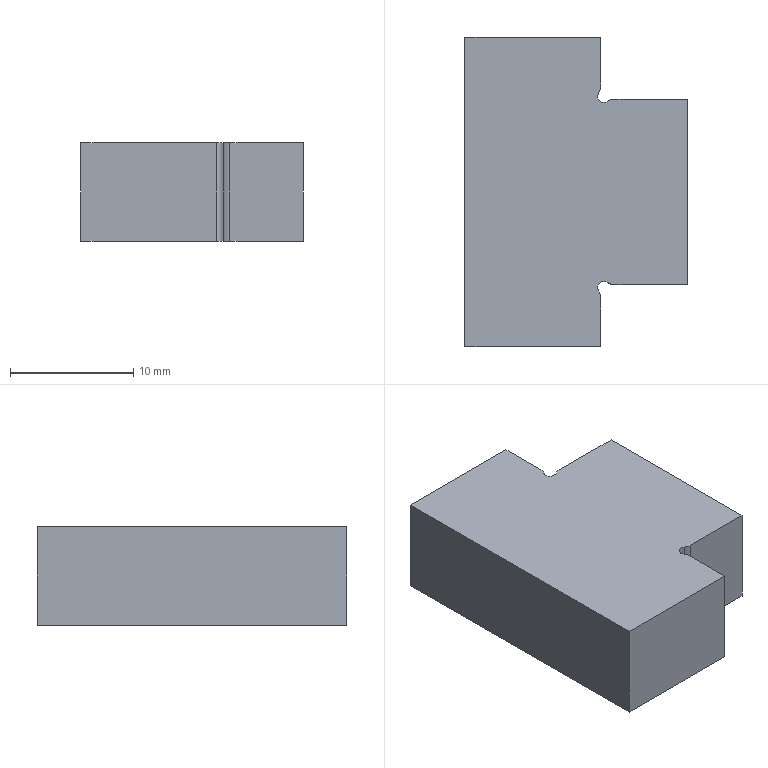Part | SolidWorks | features Fillet 1, FlatPattern 1, ICE 1, SMBaseFlange 1, SheetMetal 1 | 1 solid | 18 faces | box 18 x 25.1 x 8 mm | volume 3044 mm3 | plane 10 | cylinder 8 | commonest cylinder face diameters 1 x4 2 x4
STEP:
#1=CARTESIAN_POINT('',(4.333,12.576,8.));
#2=VERTEX_POINT('',#1);
#3=CARTESIAN_POINT('',(4.25,12.3,8.));
#4=VERTEX_POINT('',#3);
#5=CARTESIAN_POINT('',(4.75,12.3,8.));
#6=DIRECTION('',(0.,0.,1.));
#7=DIRECTION('',(1.,0.,0.));
#8=AXIS2_PLACEMENT_3D('',#5,#6,#7);
#9=CIRCLE('',#8,0.5);
#10=EDGE_CURVE('',#2,#4,#9,.T.);
#11=ORIENTED_EDGE('',*,*,#10,.T.);
#12=CARTESIAN_POINT('',(4.25,12.3,0.));
#13=VERTEX_POINT('',#12);
#14=CARTESIAN_POINT('',(4.25,12.3,0.));
#15=DIRECTION('',(0.,0.,-1.));
#16=VECTOR('',#15,1000.);
#17=LINE('',#14,#16);
#18=EDGE_CURVE('',#4,#13,#17,.T.);
#19=ORIENTED_EDGE('',*,*,#18,.T.);
#20=CARTESIAN_POINT('',(4.333,12.576,0.));
#21=VERTEX_POINT('',#20);
#22=CARTESIAN_POINT('',(4.75,12.3,0.));
#23=DIRECTION('',(0.,0.,1.));
#24=DIRECTION('',(1.,0.,0.));
#25=AXIS2_PLACEMENT_3D('',#22,#23,#24);
#26=CIRCLE('',#25,0.5);
#27=EDGE_CURVE('',#21,#13,#26,.T.);
#28=ORIENTED_EDGE('',*,*,#27,.F.);
#29=CARTESIAN_POINT('',(4.333,12.576,0.));
#30=DIRECTION('',(0.,0.,1.));
#31=VECTOR('',#30,1000.);
#32=LINE('',#29,#31);
#33=EDGE_CURVE('',#21,#2,#32,.T.);
#34=ORIENTED_EDGE('',*,*,#33,.T.);
#35=EDGE_LOOP('',(#11,#19,#28,#34));
#36=FACE_OUTER_BOUND('',#35,.T.);
#37=CARTESIAN_POINT('',(4.75,12.3,0.));
#38=DIRECTION('',(0.,0.,-1.));
#39=DIRECTION('',(-1.,0.,0.));
#40=AXIS2_PLACEMENT_3D('',#37,#38,#39);
#41=CYLINDRICAL_SURFACE('',#40,0.5);
#42=ADVANCED_FACE('',(#36),#41,.F.);
#43=CARTESIAN_POINT('',(5.026,-2.783,8.));
#44=VERTEX_POINT('',#43);
#45=CARTESIAN_POINT('',(4.25,-3.2,8.));
#46=VERTEX_POINT('',#45);
#47=CARTESIAN_POINT('',(4.75,-3.2,8.));
#48=DIRECTION('',(0.,0.,1.));
#49=DIRECTION('',(1.,0.,0.));
#50=AXIS2_PLACEMENT_3D('',#47,#48,#49);
#51=CIRCLE('',#50,0.5);
#52=EDGE_CURVE('',#44,#46,#51,.T.);
#53=ORIENTED_EDGE('',*,*,#52,.T.);
#54=CARTESIAN_POINT('',(4.25,-3.2,0.));
#55=VERTEX_POINT('',#54);
#56=CARTESIAN_POINT('',(4.25,-3.2,0.));
#57=DIRECTION('',(0.,0.,-1.));
#58=VECTOR('',#57,1000.);
#59=LINE('',#56,#58);
#60=EDGE_CURVE('',#46,#55,#59,.T.);
#61=ORIENTED_EDGE('',*,*,#60,.T.);
#62=CARTESIAN_POINT('',(5.026,-2.783,0.));
#63=VERTEX_POINT('',#62);
#64=CARTESIAN_POINT('',(4.75,-3.2,0.));
#65=DIRECTION('',(0.,0.,1.));
#66=DIRECTION('',(1.,0.,0.));
#67=AXIS2_PLACEMENT_3D('',#64,#65,#66);
#68=CIRCLE('',#67,0.5);
#69=EDGE_CURVE('',#63,#55,#68,.T.);
#70=ORIENTED_EDGE('',*,*,#69,.F.);
#71=CARTESIAN_POINT('',(5.026,-2.783,0.));
#72=DIRECTION('',(0.,0.,1.));
#73=VECTOR('',#72,1000.);
#74=LINE('',#71,#73);
#75=EDGE_CURVE('',#63,#44,#74,.T.);
#76=ORIENTED_EDGE('',*,*,#75,.T.);
#77=EDGE_LOOP('',(#53,#61,#70,#76));
#78=FACE_OUTER_BOUND('',#77,.T.);
#79=CARTESIAN_POINT('',(4.75,-3.2,0.));
#80=DIRECTION('',(0.,0.,-1.));
#81=DIRECTION('',(-1.,0.,0.));
#82=AXIS2_PLACEMENT_3D('',#79,#80,#81);
#83=CYLINDRICAL_SURFACE('',#82,0.5);
#84=ADVANCED_FACE('',(#78),#83,.F.);
#85=CARTESIAN_POINT('',(4.5,-8.,0.));
#86=VERTEX_POINT('',#85);
#87=CARTESIAN_POINT('',(4.5,-4.029,0.));
#88=VERTEX_POINT('',#87);
#89=CARTESIAN_POINT('',(4.5,-8.,0.));
#90=DIRECTION('',(0.,1.,0.));
#91=VECTOR('',#90,1000.);
#92=LINE('',#89,#91);
#93=EDGE_CURVE('',#86,#88,#92,.T.);
#94=ORIENTED_EDGE('',*,*,#93,.T.);
#95=CARTESIAN_POINT('',(4.5,-4.029,8.));
#96=VERTEX_POINT('',#95);
#97=CARTESIAN_POINT('',(4.5,-4.029,8.));
#98=DIRECTION('',(0.,0.,1.));
#99=VECTOR('',#98,1000.);
#100=LINE('',#97,#99);
#101=EDGE_CURVE('',#88,#96,#100,.T.);
#102=ORIENTED_EDGE('',*,*,#101,.T.);
#103=CARTESIAN_POINT('',(4.5,-8.,8.));
#104=VERTEX_POINT('',#103);
#105=CARTESIAN_POINT('',(4.5,-8.,8.));
#106=DIRECTION('',(0.,1.,0.));
#107=VECTOR('',#106,1000.);
#108=LINE('',#105,#107);
#109=EDGE_CURVE('',#104,#96,#108,.T.);
#110=ORIENTED_EDGE('',*,*,#109,.F.);
#111=CARTESIAN_POINT('',(4.5,-8.,8.));
#112=DIRECTION('',(0.,0.,-1.));
#113=VECTOR('',#112,1000.);
#114=LINE('',#111,#113);
#115=EDGE_CURVE('',#104,#86,#114,.T.);
#116=ORIENTED_EDGE('',*,*,#115,.T.);
#117=EDGE_LOOP('',(#94,#102,#110,#116));
#118=FACE_OUTER_BOUND('',#117,.T.);
#119=CARTESIAN_POINT('',(4.5,-8.,8.));
#120=DIRECTION('',(-1.,0.,0.));
#121=DIRECTION('',(0.,0.,1.));
#122=AXIS2_PLACEMENT_3D('',#119,#120,#121);
#123=PLANE('',#122);
#124=ADVANCED_FACE('',(#118),#123,.F.);
#125=CARTESIAN_POINT('',(5.579,-2.95,8.));
#126=VERTEX_POINT('',#125);
#127=CARTESIAN_POINT('',(11.5,-2.95,8.));
#128=VERTEX_POINT('',#127);
#129=CARTESIAN_POINT('',(4.5,-2.95,8.));
#130=DIRECTION('',(1.,0.,0.));
#131=VECTOR('',#130,1000.);
#132=LINE('',#129,#131);
#133=EDGE_CURVE('',#126,#128,#132,.T.);
#134=ORIENTED_EDGE('',*,*,#133,.F.);
#135=CARTESIAN_POINT('',(5.579,-2.95,0.));
#136=VERTEX_POINT('',#135);
#137=CARTESIAN_POINT('',(5.579,-2.95,0.));
#138=DIRECTION('',(0.,0.,-1.));
#139=VECTOR('',#138,1000.);
#140=LINE('',#137,#139);
#141=EDGE_CURVE('',#126,#136,#140,.T.);
#142=ORIENTED_EDGE('',*,*,#141,.T.);
#143=CARTESIAN_POINT('',(11.5,-2.95,0.));
#144=VERTEX_POINT('',#143);
#145=CARTESIAN_POINT('',(4.5,-2.95,0.));
#146=DIRECTION('',(1.,0.,0.));
#147=VECTOR('',#146,1000.);
#148=LINE('',#145,#147);
#149=EDGE_CURVE('',#136,#144,#148,.T.);
#150=ORIENTED_EDGE('',*,*,#149,.T.);
#151=CARTESIAN_POINT('',(11.5,-2.95,8.));
#152=DIRECTION('',(0.,0.,-1.));
#153=VECTOR('',#152,1000.);
#154=LINE('',#151,#153);
#155=EDGE_CURVE('',#128,#144,#154,.T.);
#156=ORIENTED_EDGE('',*,*,#155,.F.);
#157=EDGE_LOOP('',(#134,#142,#150,#156));
#158=FACE_OUTER_BOUND('',#157,.T.);
#159=CARTESIAN_POINT('',(4.5,-2.95,8.));
#160=DIRECTION('',(0.,1.,0.));
#161=DIRECTION('',(0.,0.,1.));
#162=AXIS2_PLACEMENT_3D('',#159,#160,#161);
#163=PLANE('',#162);
#164=ADVANCED_FACE('',(#158),#163,.F.);
#165=CARTESIAN_POINT('',(11.5,12.05,0.));
#166=VERTEX_POINT('',#165);
#167=CARTESIAN_POINT('',(5.579,12.05,0.));
#168=VERTEX_POINT('',#167);
#169=CARTESIAN_POINT('',(11.5,12.05,0.));
#170=DIRECTION('',(-1.,0.,0.));
#171=VECTOR('',#170,1000.);
#172=LINE('',#169,#171);
#173=EDGE_CURVE('',#166,#168,#172,.T.);
#174=ORIENTED_EDGE('',*,*,#173,.T.);
#175=CARTESIAN_POINT('',(5.579,12.05,8.));
#176=VERTEX_POINT('',#175);
#177=CARTESIAN_POINT('',(5.579,12.05,8.));
#178=DIRECTION('',(0.,0.,1.));
#179=VECTOR('',#178,1000.);
#180=LINE('',#177,#179);
#181=EDGE_CURVE('',#168,#176,#180,.T.);
#182=ORIENTED_EDGE('',*,*,#181,.T.);
#183=CARTESIAN_POINT('',(11.5,12.05,8.));
#184=VERTEX_POINT('',#183);
#185=CARTESIAN_POINT('',(11.5,12.05,8.));
#186=DIRECTION('',(-1.,0.,0.));
#187=VECTOR('',#186,1000.);
#188=LINE('',#185,#187);
#189=EDGE_CURVE('',#184,#176,#188,.T.);
#190=ORIENTED_EDGE('',*,*,#189,.F.);
#191=CARTESIAN_POINT('',(11.5,12.05,8.));
#192=DIRECTION('',(0.,0.,-1.));
#193=VECTOR('',#192,1000.);
#194=LINE('',#191,#193);
#195=EDGE_CURVE('',#184,#166,#194,.T.);
#196=ORIENTED_EDGE('',*,*,#195,.T.);
#197=EDGE_LOOP('',(#174,#182,#190,#196));
#198=FACE_OUTER_BOUND('',#197,.T.);
#199=CARTESIAN_POINT('',(11.5,12.05,8.));
#200=DIRECTION('',(0.,-1.,0.));
#201=DIRECTION('',(1.,0.,0.));
#202=AXIS2_PLACEMENT_3D('',#199,#200,#201);
#203=PLANE('',#202);
#204=ADVANCED_FACE('',(#198),#203,.F.);
#205=CARTESIAN_POINT('',(4.5,13.129,8.));
#206=VERTEX_POINT('',#205);
#207=CARTESIAN_POINT('',(4.5,17.1,8.));
#208=VERTEX_POINT('',#207);
#209=CARTESIAN_POINT('',(4.5,12.05,8.));
#210=DIRECTION('',(0.,1.,0.));
#211=VECTOR('',#210,1000.);
#212=LINE('',#209,#211);
#213=EDGE_CURVE('',#206,#208,#212,.T.);
#214=ORIENTED_EDGE('',*,*,#213,.F.);
#215=CARTESIAN_POINT('',(4.5,13.129,0.));
#216=VERTEX_POINT('',#215);
#217=CARTESIAN_POINT('',(4.5,13.129,0.));
#218=DIRECTION('',(0.,0.,-1.));
#219=VECTOR('',#218,1000.);
#220=LINE('',#217,#219);
#221=EDGE_CURVE('',#206,#216,#220,.T.);
#222=ORIENTED_EDGE('',*,*,#221,.T.);
#223=CARTESIAN_POINT('',(4.5,17.1,0.));
#224=VERTEX_POINT('',#223);
#225=CARTESIAN_POINT('',(4.5,12.05,0.));
#226=DIRECTION('',(0.,1.,0.));
#227=VECTOR('',#226,1000.);
#228=LINE('',#225,#227);
#229=EDGE_CURVE('',#216,#224,#228,.T.);
#230=ORIENTED_EDGE('',*,*,#229,.T.);
#231=CARTESIAN_POINT('',(4.5,17.1,8.));
#232=DIRECTION('',(0.,0.,-1.));
#233=VECTOR('',#232,1000.);
#234=LINE('',#231,#233);
#235=EDGE_CURVE('',#208,#224,#234,.T.);
#236=ORIENTED_EDGE('',*,*,#235,.F.);
#237=EDGE_LOOP('',(#214,#222,#230,#236));
#238=FACE_OUTER_BOUND('',#237,.T.);
#239=CARTESIAN_POINT('',(4.5,12.05,8.));
#240=DIRECTION('',(-1.,0.,0.));
#241=DIRECTION('',(0.,0.,1.));
#242=AXIS2_PLACEMENT_3D('',#239,#240,#241);
#243=PLANE('',#242);
#244=ADVANCED_FACE('',(#238),#243,.F.);
#245=CARTESIAN_POINT('',(-6.5,17.1,0.));
#246=VERTEX_POINT('',#245);
#247=CARTESIAN_POINT('',(-6.5,-8.,0.));
#248=VERTEX_POINT('',#247);
#249=CARTESIAN_POINT('',(-6.5,-8.,0.));
#250=DIRECTION('',(0.,-1.,0.));
#251=VECTOR('',#250,1000.);
#252=LINE('',#249,#251);
#253=EDGE_CURVE('',#246,#248,#252,.T.);
#254=ORIENTED_EDGE('',*,*,#253,.T.);
#255=CARTESIAN_POINT('',(-6.5,-8.,8.));
#256=VERTEX_POINT('',#255);
#257=CARTESIAN_POINT('',(-6.5,-8.,8.));
#258=DIRECTION('',(0.,0.,-1.));
#259=VECTOR('',#258,1000.);
#260=LINE('',#257,#259);
#261=EDGE_CURVE('',#256,#248,#260,.T.);
#262=ORIENTED_EDGE('',*,*,#261,.F.);
#263=CARTESIAN_POINT('',(-6.5,17.1,8.));
#264=VERTEX_POINT('',#263);
#265=CARTESIAN_POINT('',(-6.5,-8.,8.));
#266=DIRECTION('',(0.,-1.,0.));
#267=VECTOR('',#266,1000.);
#268=LINE('',#265,#267);
#269=EDGE_CURVE('',#264,#256,#268,.T.);
#270=ORIENTED_EDGE('',*,*,#269,.F.);
#271=CARTESIAN_POINT('',(-6.5,17.1,8.));
#272=DIRECTION('',(0.,0.,-1.));
#273=VECTOR('',#272,1000.);
#274=LINE('',#271,#273);
#275=EDGE_CURVE('',#264,#246,#274,.T.);
#276=ORIENTED_EDGE('',*,*,#275,.T.);
#277=EDGE_LOOP('',(#254,#262,#270,#276));
#278=FACE_OUTER_BOUND('',#277,.T.);
#279=CARTESIAN_POINT('',(-6.5,-8.,8.));
#280=DIRECTION('',(1.,0.,0.));
#281=DIRECTION('',(0.,0.,-1.));
#282=AXIS2_PLACEMENT_3D('',#279,#280,#281);
#283=PLANE('',#282);
#284=ADVANCED_FACE('',(#278),#283,.F.);
#285=CARTESIAN_POINT('',(-6.5,-8.,0.));
#286=DIRECTION('',(1.,0.,0.));
#287=VECTOR('',#286,1000.);
#288=LINE('',#285,#287);
#289=EDGE_CURVE('',#248,#86,#288,.T.);
#290=ORIENTED_EDGE('',*,*,#289,.T.);
#291=ORIENTED_EDGE('',*,*,#115,.F.);
#292=CARTESIAN_POINT('',(-6.5,-8.,8.));
#293=DIRECTION('',(1.,0.,0.));
#294=VECTOR('',#293,1000.);
#295=LINE('',#292,#294);
#296=EDGE_CURVE('',#256,#104,#295,.T.);
#297=ORIENTED_EDGE('',*,*,#296,.F.);
#298=ORIENTED_EDGE('',*,*,#261,.T.);
#299=EDGE_LOOP('',(#290,#291,#297,#298));
#300=FACE_OUTER_BOUND('',#299,.T.);
#301=CARTESIAN_POINT('',(-6.5,-8.,8.));
#302=DIRECTION('',(0.,1.,0.));
#303=DIRECTION('',(0.,0.,1.));
#304=AXIS2_PLACEMENT_3D('',#301,#302,#303);
#305=PLANE('',#304);
#306=ADVANCED_FACE('',(#300),#305,.F.);
#307=CARTESIAN_POINT('',(11.5,-2.95,0.));
#308=DIRECTION('',(0.,1.,0.));
#309=VECTOR('',#308,1000.);
#310=LINE('',#307,#309);
#311=EDGE_CURVE('',#144,#166,#310,.T.);
#312=ORIENTED_EDGE('',*,*,#311,.T.);
#313=ORIENTED_EDGE('',*,*,#195,.F.);
#314=CARTESIAN_POINT('',(11.5,-2.95,8.));
#315=DIRECTION('',(0.,1.,0.));
#316=VECTOR('',#315,1000.);
#317=LINE('',#314,#316);
#318=EDGE_CURVE('',#128,#184,#317,.T.);
#319=ORIENTED_EDGE('',*,*,#318,.F.);
#320=ORIENTED_EDGE('',*,*,#155,.T.);
#321=EDGE_LOOP('',(#312,#313,#319,#320));
#322=FACE_OUTER_BOUND('',#321,.T.);
#323=CARTESIAN_POINT('',(11.5,-2.95,8.));
#324=DIRECTION('',(-1.,0.,0.));
#325=DIRECTION('',(0.,0.,1.));
#326=AXIS2_PLACEMENT_3D('',#323,#324,#325);
#327=PLANE('',#326);
#328=ADVANCED_FACE('',(#322),#327,.F.);
#329=CARTESIAN_POINT('',(-6.5,17.1,0.));
#330=DIRECTION('',(-1.,0.,0.));
#331=VECTOR('',#330,1000.);
#332=LINE('',#329,#331);
#333=EDGE_CURVE('',#224,#246,#332,.T.);
#334=ORIENTED_EDGE('',*,*,#333,.T.);
#335=ORIENTED_EDGE('',*,*,#275,.F.);
#336=CARTESIAN_POINT('',(-6.5,17.1,8.));
#337=DIRECTION('',(-1.,0.,0.));
#338=VECTOR('',#337,1000.);
#339=LINE('',#336,#338);
#340=EDGE_CURVE('',#208,#264,#339,.T.);
#341=ORIENTED_EDGE('',*,*,#340,.F.);
#342=ORIENTED_EDGE('',*,*,#235,.T.);
#343=EDGE_LOOP('',(#334,#335,#341,#342));
#344=FACE_OUTER_BOUND('',#343,.T.);
#345=CARTESIAN_POINT('',(-6.5,17.1,8.));
#346=DIRECTION('',(0.,-1.,0.));
#347=DIRECTION('',(0.,0.,-1.));
#348=AXIS2_PLACEMENT_3D('',#345,#346,#347);
#349=PLANE('',#348);
#350=ADVANCED_FACE('',(#344),#349,.F.);
#351=ORIENTED_EDGE('',*,*,#189,.T.);
#352=CARTESIAN_POINT('',(5.026,11.883,8.));
#353=VERTEX_POINT('',#352);
#354=CARTESIAN_POINT('',(5.579,11.05,8.));
#355=DIRECTION('',(0.,0.,1.));
#356=DIRECTION('',(-1.,0.,0.));
#357=AXIS2_PLACEMENT_3D('',#354,#355,#356);
#358=CIRCLE('',#357,1.);
#359=EDGE_CURVE('',#176,#353,#358,.T.);
#360=ORIENTED_EDGE('',*,*,#359,.T.);
#361=CARTESIAN_POINT('',(4.75,12.3,8.));
#362=DIRECTION('',(0.,0.,1.));
#363=DIRECTION('',(1.,0.,0.));
#364=AXIS2_PLACEMENT_3D('',#361,#362,#363);
#365=CIRCLE('',#364,0.5);
#366=EDGE_CURVE('',#4,#353,#365,.T.);
#367=ORIENTED_EDGE('',*,*,#366,.F.);
#368=ORIENTED_EDGE('',*,*,#10,.F.);
#369=CARTESIAN_POINT('',(3.5,13.129,8.));
#370=DIRECTION('',(0.,0.,1.));
#371=DIRECTION('',(-1.,0.,0.));
#372=AXIS2_PLACEMENT_3D('',#369,#370,#371);
#373=CIRCLE('',#372,1.);
#374=EDGE_CURVE('',#2,#206,#373,.T.);
#375=ORIENTED_EDGE('',*,*,#374,.T.);
#376=ORIENTED_EDGE('',*,*,#213,.T.);
#377=ORIENTED_EDGE('',*,*,#340,.T.);
#378=ORIENTED_EDGE('',*,*,#269,.T.);
#379=ORIENTED_EDGE('',*,*,#296,.T.);
#380=ORIENTED_EDGE('',*,*,#109,.T.);
#381=CARTESIAN_POINT('',(4.333,-3.476,8.));
#382=VERTEX_POINT('',#381);
#383=CARTESIAN_POINT('',(3.5,-4.029,8.));
#384=DIRECTION('',(0.,0.,1.));
#385=DIRECTION('',(-1.,0.,0.));
#386=AXIS2_PLACEMENT_3D('',#383,#384,#385);
#387=CIRCLE('',#386,1.);
#388=EDGE_CURVE('',#96,#382,#387,.T.);
#389=ORIENTED_EDGE('',*,*,#388,.T.);
#390=CARTESIAN_POINT('',(4.75,-3.2,8.));
#391=DIRECTION('',(0.,0.,1.));
#392=DIRECTION('',(1.,0.,0.));
#393=AXIS2_PLACEMENT_3D('',#390,#391,#392);
#394=CIRCLE('',#393,0.5);
#395=EDGE_CURVE('',#46,#382,#394,.T.);
#396=ORIENTED_EDGE('',*,*,#395,.F.);
#397=ORIENTED_EDGE('',*,*,#52,.F.);
#398=CARTESIAN_POINT('',(5.579,-1.95,8.));
#399=DIRECTION('',(0.,0.,1.));
#400=DIRECTION('',(-1.,0.,0.));
#401=AXIS2_PLACEMENT_3D('',#398,#399,#400);
#402=CIRCLE('',#401,1.);
#403=EDGE_CURVE('',#44,#126,#402,.T.);
#404=ORIENTED_EDGE('',*,*,#403,.T.);
#405=ORIENTED_EDGE('',*,*,#133,.T.);
#406=ORIENTED_EDGE('',*,*,#318,.T.);
#407=EDGE_LOOP('',(#351,#360,#367,#368,#375,#376,#377,#378,#379,#380,#389,#396,#397,#404,#405,#406));
#408=FACE_OUTER_BOUND('',#407,.T.);
#409=CARTESIAN_POINT('',(0.,0.,8.));
#410=DIRECTION('',(0.,0.,-1.));
#411=DIRECTION('',(-1.,0.,0.));
#412=AXIS2_PLACEMENT_3D('',#409,#410,#411);
#413=PLANE('',#412);
#414=ADVANCED_FACE('',(#408),#413,.F.);
#415=ORIENTED_EDGE('',*,*,#27,.T.);
#416=CARTESIAN_POINT('',(5.026,11.883,0.));
#417=VERTEX_POINT('',#416);
#418=CARTESIAN_POINT('',(4.75,12.3,0.));
#419=DIRECTION('',(0.,0.,1.));
#420=DIRECTION('',(1.,0.,0.));
#421=AXIS2_PLACEMENT_3D('',#418,#419,#420);
#422=CIRCLE('',#421,0.5);
#423=EDGE_CURVE('',#13,#417,#422,.T.);
#424=ORIENTED_EDGE('',*,*,#423,.T.);
#425=CARTESIAN_POINT('',(5.579,11.05,0.));
#426=DIRECTION('',(0.,0.,-1.));
#427=DIRECTION('',(-1.,0.,0.));
#428=AXIS2_PLACEMENT_3D('',#425,#426,#427);
#429=CIRCLE('',#428,1.);
#430=EDGE_CURVE('',#417,#168,#429,.T.);
#431=ORIENTED_EDGE('',*,*,#430,.T.);
#432=ORIENTED_EDGE('',*,*,#173,.F.);
#433=ORIENTED_EDGE('',*,*,#311,.F.);
#434=ORIENTED_EDGE('',*,*,#149,.F.);
#435=CARTESIAN_POINT('',(5.579,-1.95,0.));
#436=DIRECTION('',(0.,0.,-1.));
#437=DIRECTION('',(-1.,0.,0.));
#438=AXIS2_PLACEMENT_3D('',#435,#436,#437);
#439=CIRCLE('',#438,1.);
#440=EDGE_CURVE('',#136,#63,#439,.T.);
#441=ORIENTED_EDGE('',*,*,#440,.T.);
#442=ORIENTED_EDGE('',*,*,#69,.T.);
#443=CARTESIAN_POINT('',(4.333,-3.476,0.));
#444=VERTEX_POINT('',#443);
#445=CARTESIAN_POINT('',(4.75,-3.2,0.));
#446=DIRECTION('',(0.,0.,1.));
#447=DIRECTION('',(1.,0.,0.));
#448=AXIS2_PLACEMENT_3D('',#445,#446,#447);
#449=CIRCLE('',#448,0.5);
#450=EDGE_CURVE('',#55,#444,#449,.T.);
#451=ORIENTED_EDGE('',*,*,#450,.T.);
#452=CARTESIAN_POINT('',(3.5,-4.029,0.));
#453=DIRECTION('',(0.,0.,-1.));
#454=DIRECTION('',(-1.,0.,0.));
#455=AXIS2_PLACEMENT_3D('',#452,#453,#454);
#456=CIRCLE('',#455,1.);
#457=EDGE_CURVE('',#444,#88,#456,.T.);
#458=ORIENTED_EDGE('',*,*,#457,.T.);
#459=ORIENTED_EDGE('',*,*,#93,.F.);
#460=ORIENTED_EDGE('',*,*,#289,.F.);
#461=ORIENTED_EDGE('',*,*,#253,.F.);
#462=ORIENTED_EDGE('',*,*,#333,.F.);
#463=ORIENTED_EDGE('',*,*,#229,.F.);
#464=CARTESIAN_POINT('',(3.5,13.129,0.));
#465=DIRECTION('',(0.,0.,-1.));
#466=DIRECTION('',(-1.,0.,0.));
#467=AXIS2_PLACEMENT_3D('',#464,#465,#466);
#468=CIRCLE('',#467,1.);
#469=EDGE_CURVE('',#216,#21,#468,.T.);
#470=ORIENTED_EDGE('',*,*,#469,.T.);
#471=EDGE_LOOP('',(#415,#424,#431,#432,#433,#434,#441,#442,#451,#458,#459,#460,#461,#462,#463,#470));
#472=FACE_OUTER_BOUND('',#471,.T.);
#473=CARTESIAN_POINT('',(0.,0.,0.));
#474=DIRECTION('',(0.,0.,-1.));
#475=DIRECTION('',(-1.,0.,0.));
#476=AXIS2_PLACEMENT_3D('',#473,#474,#475);
#477=PLANE('',#476);
#478=ADVANCED_FACE('',(#472),#477,.T.);
#479=ORIENTED_EDGE('',*,*,#60,.F.);
#480=ORIENTED_EDGE('',*,*,#395,.T.);
#481=CARTESIAN_POINT('',(4.333,-3.476,0.));
#482=DIRECTION('',(0.,0.,-1.));
#483=VECTOR('',#482,1000.);
#484=LINE('',#481,#483);
#485=EDGE_CURVE('',#382,#444,#484,.T.);
#486=ORIENTED_EDGE('',*,*,#485,.T.);
#487=ORIENTED_EDGE('',*,*,#450,.F.);
#488=EDGE_LOOP('',(#479,#480,#486,#487));
#489=FACE_OUTER_BOUND('',#488,.T.);
#490=CARTESIAN_POINT('',(4.75,-3.2,0.));
#491=DIRECTION('',(0.,0.,-1.));
#492=DIRECTION('',(-1.,0.,0.));
#493=AXIS2_PLACEMENT_3D('',#490,#491,#492);
#494=CYLINDRICAL_SURFACE('',#493,0.5);
#495=ADVANCED_FACE('',(#489),#494,.F.);
#496=ORIENTED_EDGE('',*,*,#18,.F.);
#497=ORIENTED_EDGE('',*,*,#366,.T.);
#498=CARTESIAN_POINT('',(5.026,11.883,0.));
#499=DIRECTION('',(0.,0.,-1.));
#500=VECTOR('',#499,1000.);
#501=LINE('',#498,#500);
#502=EDGE_CURVE('',#353,#417,#501,.T.);
#503=ORIENTED_EDGE('',*,*,#502,.T.);
#504=ORIENTED_EDGE('',*,*,#423,.F.);
#505=EDGE_LOOP('',(#496,#497,#503,#504));
#506=FACE_OUTER_BOUND('',#505,.T.);
#507=CARTESIAN_POINT('',(4.75,12.3,0.));
#508=DIRECTION('',(0.,0.,-1.));
#509=DIRECTION('',(-1.,0.,0.));
#510=AXIS2_PLACEMENT_3D('',#507,#508,#509);
#511=CYLINDRICAL_SURFACE('',#510,0.5);
#512=ADVANCED_FACE('',(#506),#511,.F.);
#513=ORIENTED_EDGE('',*,*,#430,.F.);
#514=ORIENTED_EDGE('',*,*,#502,.F.);
#515=ORIENTED_EDGE('',*,*,#359,.F.);
#516=ORIENTED_EDGE('',*,*,#181,.F.);
#517=EDGE_LOOP('',(#513,#514,#515,#516));
#518=FACE_OUTER_BOUND('',#517,.T.);
#519=CARTESIAN_POINT('',(5.579,11.05,0.));
#520=DIRECTION('',(0.,0.,-1.));
#521=DIRECTION('',(-1.,0.,0.));
#522=AXIS2_PLACEMENT_3D('',#519,#520,#521);
#523=CYLINDRICAL_SURFACE('',#522,1.);
#524=ADVANCED_FACE('',(#518),#523,.T.);
#525=ORIENTED_EDGE('',*,*,#469,.F.);
#526=ORIENTED_EDGE('',*,*,#221,.F.);
#527=ORIENTED_EDGE('',*,*,#374,.F.);
#528=ORIENTED_EDGE('',*,*,#33,.F.);
#529=EDGE_LOOP('',(#525,#526,#527,#528));
#530=FACE_OUTER_BOUND('',#529,.T.);
#531=CARTESIAN_POINT('',(3.5,13.129,0.));
#532=DIRECTION('',(0.,0.,-1.));
#533=DIRECTION('',(-1.,0.,0.));
#534=AXIS2_PLACEMENT_3D('',#531,#532,#533);
#535=CYLINDRICAL_SURFACE('',#534,1.);
#536=ADVANCED_FACE('',(#530),#535,.T.);
#537=ORIENTED_EDGE('',*,*,#440,.F.);
#538=ORIENTED_EDGE('',*,*,#141,.F.);
#539=ORIENTED_EDGE('',*,*,#403,.F.);
#540=ORIENTED_EDGE('',*,*,#75,.F.);
#541=EDGE_LOOP('',(#537,#538,#539,#540));
#542=FACE_OUTER_BOUND('',#541,.T.);
#543=CARTESIAN_POINT('',(5.579,-1.95,0.));
#544=DIRECTION('',(0.,0.,-1.));
#545=DIRECTION('',(-1.,0.,0.));
#546=AXIS2_PLACEMENT_3D('',#543,#544,#545);
#547=CYLINDRICAL_SURFACE('',#546,1.);
#548=ADVANCED_FACE('',(#542),#547,.T.);
#549=ORIENTED_EDGE('',*,*,#457,.F.);
#550=ORIENTED_EDGE('',*,*,#485,.F.);
#551=ORIENTED_EDGE('',*,*,#388,.F.);
#552=ORIENTED_EDGE('',*,*,#101,.F.);
#553=EDGE_LOOP('',(#549,#550,#551,#552));
#554=FACE_OUTER_BOUND('',#553,.T.);
#555=CARTESIAN_POINT('',(3.5,-4.029,0.));
#556=DIRECTION('',(0.,0.,-1.));
#557=DIRECTION('',(-1.,0.,0.));
#558=AXIS2_PLACEMENT_3D('',#555,#556,#557);
#559=CYLINDRICAL_SURFACE('',#558,1.);
#560=ADVANCED_FACE('',(#554),#559,.T.);
#561=CLOSED_SHELL('',(#42,#84,#124,#164,#204,#244,#284,#306,#328,#350,#414,#478,#495,#512,#524,#536,#548,#560));
#562=MANIFOLD_SOLID_BREP('',#561);
#563=CARTESIAN_POINT('',(0.,0.,0.));
#564=DIRECTION('',(0.,0.,1.));
#565=DIRECTION('',(1.,0.,0.));
#566=AXIS2_PLACEMENT_3D('',#563,#564,#565);
#567=(LENGTH_UNIT()NAMED_UNIT(*)SI_UNIT(.MILLI.,.METRE.));
#568=UNCERTAINTY_MEASURE_WITH_UNIT(LENGTH_MEASURE(0.00001),#567,'','');
#569=(NAMED_UNIT(*)PLANE_ANGLE_UNIT()SI_UNIT($,.RADIAN.));
#570=(NAMED_UNIT(*)SI_UNIT($,.STERADIAN.)SOLID_ANGLE_UNIT());
#571=(GEOMETRIC_REPRESENTATION_CONTEXT(3)GLOBAL_UNCERTAINTY_ASSIGNED_CONTEXT((#568))GLOBAL_UNIT_ASSIGNED_CONTEXT((#567,#569,#570))REPRESENTATION_CONTEXT('',''));
#572=ADVANCED_BREP_SHAPE_REPRESENTATION('',(#562,#566),#571);